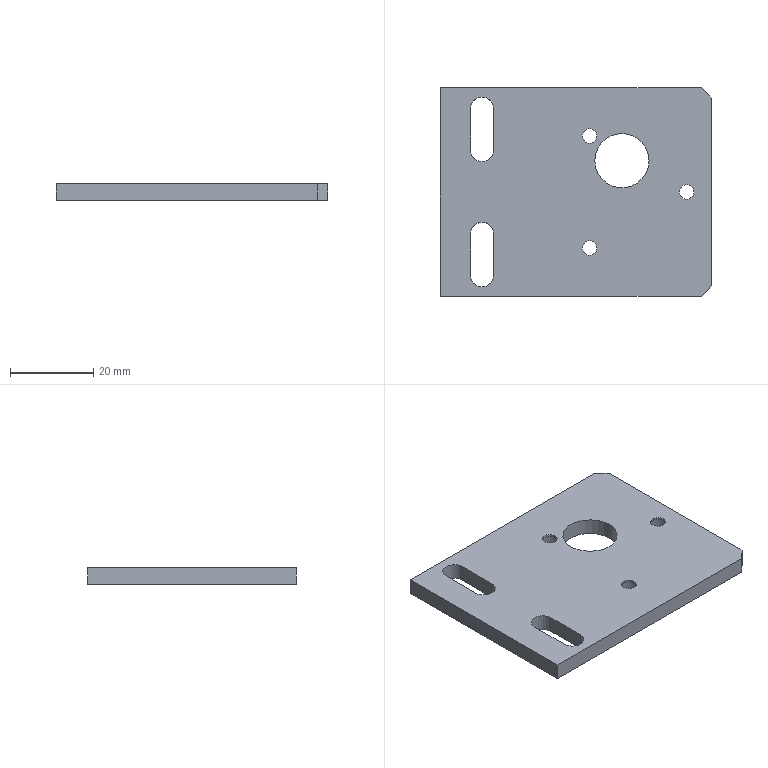Part | SolidWorks | features BaseBody 1 | 1 solid | 33 faces | box 65 x 50 x 4 mm | volume 11503 mm3 | cylinder 18 | plane 15 | commonest cylinder face diameters 3.5 x6 6 x6 5.5 x4 13 x2
STEP:
#1=CARTESIAN_POINT('',(41.797,20.428,0.));
#2=VERTEX_POINT('',#1);
#3=CARTESIAN_POINT('',(54.797,20.428,0.));
#4=VERTEX_POINT('',#3);
#5=CARTESIAN_POINT('',(48.297,20.428,0.));
#6=DIRECTION('',(0.,0.,1.));
#7=DIRECTION('',(1.,0.,0.));
#8=AXIS2_PLACEMENT_3D('',#5,#6,#7);
#9=CIRCLE('',#8,6.5);
#10=EDGE_CURVE('',#2,#4,#9,.T.);
#11=ORIENTED_EDGE('',*,*,#10,.F.);
#12=CARTESIAN_POINT('',(41.797,20.428,4.));
#13=VERTEX_POINT('',#12);
#14=CARTESIAN_POINT('',(41.797,20.428,-78.104));
#15=DIRECTION('',(0.,0.,1.));
#16=VECTOR('',#15,1000.);
#17=LINE('',#14,#16);
#18=EDGE_CURVE('',#2,#13,#17,.T.);
#19=ORIENTED_EDGE('',*,*,#18,.T.);
#20=CARTESIAN_POINT('',(54.797,20.428,4.));
#21=VERTEX_POINT('',#20);
#22=CARTESIAN_POINT('',(48.297,20.428,4.));
#23=DIRECTION('',(0.,0.,-1.));
#24=DIRECTION('',(1.,0.,0.));
#25=AXIS2_PLACEMENT_3D('',#22,#23,#24);
#26=CIRCLE('',#25,6.5);
#27=EDGE_CURVE('',#21,#13,#26,.T.);
#28=ORIENTED_EDGE('',*,*,#27,.F.);
#29=CARTESIAN_POINT('',(54.797,20.428,-78.104));
#30=DIRECTION('',(0.,0.,1.));
#31=VECTOR('',#30,1000.);
#32=LINE('',#29,#31);
#33=EDGE_CURVE('',#4,#21,#32,.T.);
#34=ORIENTED_EDGE('',*,*,#33,.F.);
#35=EDGE_LOOP('',(#11,#19,#28,#34));
#36=FACE_OUTER_BOUND('',#35,.T.);
#37=CARTESIAN_POINT('',(48.297,20.428,-78.104));
#38=DIRECTION('',(0.,0.,1.));
#39=DIRECTION('',(1.,0.,0.));
#40=AXIS2_PLACEMENT_3D('',#37,#38,#39);
#41=CYLINDRICAL_SURFACE('',#40,6.5);
#42=ADVANCED_FACE('',(#36),#41,.F.);
#43=CARTESIAN_POINT('',(42.297,26.328,4.));
#44=VERTEX_POINT('',#43);
#45=CARTESIAN_POINT('',(38.797,26.328,4.));
#46=VERTEX_POINT('',#45);
#47=CARTESIAN_POINT('',(40.547,26.328,4.));
#48=DIRECTION('',(0.,0.,-1.));
#49=DIRECTION('',(-1.,0.,0.));
#50=AXIS2_PLACEMENT_3D('',#47,#48,#49);
#51=CIRCLE('',#50,1.75);
#52=EDGE_CURVE('',#44,#46,#51,.T.);
#53=ORIENTED_EDGE('',*,*,#52,.F.);
#54=CARTESIAN_POINT('',(42.297,26.328,3.5));
#55=VERTEX_POINT('',#54);
#56=CARTESIAN_POINT('',(42.297,26.328,82.104));
#57=DIRECTION('',(0.,0.,-1.));
#58=VECTOR('',#57,1000.);
#59=LINE('',#56,#58);
#60=EDGE_CURVE('',#44,#55,#59,.T.);
#61=ORIENTED_EDGE('',*,*,#60,.T.);
#62=CARTESIAN_POINT('',(38.797,26.328,3.5));
#63=VERTEX_POINT('',#62);
#64=CARTESIAN_POINT('',(40.547,26.328,3.5));
#65=DIRECTION('',(0.,0.,1.));
#66=DIRECTION('',(-1.,0.,0.));
#67=AXIS2_PLACEMENT_3D('',#64,#65,#66);
#68=CIRCLE('',#67,1.75);
#69=EDGE_CURVE('',#63,#55,#68,.T.);
#70=ORIENTED_EDGE('',*,*,#69,.F.);
#71=CARTESIAN_POINT('',(38.797,26.328,82.104));
#72=DIRECTION('',(0.,0.,-1.));
#73=VECTOR('',#72,1000.);
#74=LINE('',#71,#73);
#75=EDGE_CURVE('',#46,#63,#74,.T.);
#76=ORIENTED_EDGE('',*,*,#75,.F.);
#77=EDGE_LOOP('',(#53,#61,#70,#76));
#78=FACE_OUTER_BOUND('',#77,.T.);
#79=CARTESIAN_POINT('',(40.547,26.328,82.104));
#80=DIRECTION('',(0.,0.,-1.));
#81=DIRECTION('',(-1.,0.,0.));
#82=AXIS2_PLACEMENT_3D('',#79,#80,#81);
#83=CYLINDRICAL_SURFACE('',#82,1.75);
#84=ADVANCED_FACE('',(#78),#83,.F.);
#85=CARTESIAN_POINT('',(42.297,-0.4722,4.));
#86=VERTEX_POINT('',#85);
#87=CARTESIAN_POINT('',(38.797,-0.4722,4.));
#88=VERTEX_POINT('',#87);
#89=CARTESIAN_POINT('',(40.547,-0.4722,4.));
#90=DIRECTION('',(0.,0.,-1.));
#91=DIRECTION('',(-1.,0.,0.));
#92=AXIS2_PLACEMENT_3D('',#89,#90,#91);
#93=CIRCLE('',#92,1.75);
#94=EDGE_CURVE('',#86,#88,#93,.T.);
#95=ORIENTED_EDGE('',*,*,#94,.F.);
#96=CARTESIAN_POINT('',(42.297,-0.4722,3.5));
#97=VERTEX_POINT('',#96);
#98=CARTESIAN_POINT('',(42.297,-0.4722,82.104));
#99=DIRECTION('',(0.,0.,-1.));
#100=VECTOR('',#99,1000.);
#101=LINE('',#98,#100);
#102=EDGE_CURVE('',#86,#97,#101,.T.);
#103=ORIENTED_EDGE('',*,*,#102,.T.);
#104=CARTESIAN_POINT('',(38.797,-0.4722,3.5));
#105=VERTEX_POINT('',#104);
#106=CARTESIAN_POINT('',(40.547,-0.4722,3.5));
#107=DIRECTION('',(0.,0.,1.));
#108=DIRECTION('',(-1.,0.,0.));
#109=AXIS2_PLACEMENT_3D('',#106,#107,#108);
#110=CIRCLE('',#109,1.75);
#111=EDGE_CURVE('',#105,#97,#110,.T.);
#112=ORIENTED_EDGE('',*,*,#111,.F.);
#113=CARTESIAN_POINT('',(38.797,-0.4722,82.104));
#114=DIRECTION('',(0.,0.,-1.));
#115=VECTOR('',#114,1000.);
#116=LINE('',#113,#115);
#117=EDGE_CURVE('',#88,#105,#116,.T.);
#118=ORIENTED_EDGE('',*,*,#117,.F.);
#119=EDGE_LOOP('',(#95,#103,#112,#118));
#120=FACE_OUTER_BOUND('',#119,.T.);
#121=CARTESIAN_POINT('',(40.547,-0.4722,82.104));
#122=DIRECTION('',(0.,0.,-1.));
#123=DIRECTION('',(-1.,0.,0.));
#124=AXIS2_PLACEMENT_3D('',#121,#122,#123);
#125=CYLINDRICAL_SURFACE('',#124,1.75);
#126=ADVANCED_FACE('',(#120),#125,.F.);
#127=CARTESIAN_POINT('',(65.547,12.928,4.));
#128=VERTEX_POINT('',#127);
#129=CARTESIAN_POINT('',(62.047,12.928,4.));
#130=VERTEX_POINT('',#129);
#131=CARTESIAN_POINT('',(63.797,12.928,4.));
#132=DIRECTION('',(0.,0.,-1.));
#133=DIRECTION('',(-1.,0.,0.));
#134=AXIS2_PLACEMENT_3D('',#131,#132,#133);
#135=CIRCLE('',#134,1.75);
#136=EDGE_CURVE('',#128,#130,#135,.T.);
#137=ORIENTED_EDGE('',*,*,#136,.F.);
#138=CARTESIAN_POINT('',(65.547,12.928,3.5));
#139=VERTEX_POINT('',#138);
#140=CARTESIAN_POINT('',(65.547,12.928,82.104));
#141=DIRECTION('',(0.,0.,-1.));
#142=VECTOR('',#141,1000.);
#143=LINE('',#140,#142);
#144=EDGE_CURVE('',#128,#139,#143,.T.);
#145=ORIENTED_EDGE('',*,*,#144,.T.);
#146=CARTESIAN_POINT('',(62.047,12.928,3.5));
#147=VERTEX_POINT('',#146);
#148=CARTESIAN_POINT('',(63.797,12.928,3.5));
#149=DIRECTION('',(0.,0.,1.));
#150=DIRECTION('',(-1.,0.,0.));
#151=AXIS2_PLACEMENT_3D('',#148,#149,#150);
#152=CIRCLE('',#151,1.75);
#153=EDGE_CURVE('',#147,#139,#152,.T.);
#154=ORIENTED_EDGE('',*,*,#153,.F.);
#155=CARTESIAN_POINT('',(62.047,12.928,82.104));
#156=DIRECTION('',(0.,0.,-1.));
#157=VECTOR('',#156,1000.);
#158=LINE('',#155,#157);
#159=EDGE_CURVE('',#130,#147,#158,.T.);
#160=ORIENTED_EDGE('',*,*,#159,.F.);
#161=EDGE_LOOP('',(#137,#145,#154,#160));
#162=FACE_OUTER_BOUND('',#161,.T.);
#163=CARTESIAN_POINT('',(63.797,12.928,82.104));
#164=DIRECTION('',(0.,0.,-1.));
#165=DIRECTION('',(-1.,0.,0.));
#166=AXIS2_PLACEMENT_3D('',#163,#164,#165);
#167=CYLINDRICAL_SURFACE('',#166,1.75);
#168=ADVANCED_FACE('',(#162),#167,.F.);
#169=CARTESIAN_POINT('',(43.547,26.328,3.5));
#170=VERTEX_POINT('',#169);
#171=CARTESIAN_POINT('',(37.547,26.328,3.5));
#172=VERTEX_POINT('',#171);
#173=CARTESIAN_POINT('',(40.547,26.328,3.5));
#174=DIRECTION('',(0.,0.,-1.));
#175=DIRECTION('',(-1.,0.,0.));
#176=AXIS2_PLACEMENT_3D('',#173,#174,#175);
#177=CIRCLE('',#176,3.);
#178=EDGE_CURVE('',#170,#172,#177,.T.);
#179=ORIENTED_EDGE('',*,*,#178,.F.);
#180=CARTESIAN_POINT('',(43.547,26.328,0.));
#181=VERTEX_POINT('',#180);
#182=CARTESIAN_POINT('',(43.547,26.328,1.75));
#183=DIRECTION('',(0.,0.,-1.));
#184=VECTOR('',#183,1000.);
#185=LINE('',#182,#184);
#186=EDGE_CURVE('',#170,#181,#185,.T.);
#187=ORIENTED_EDGE('',*,*,#186,.T.);
#188=CARTESIAN_POINT('',(37.547,26.328,0.));
#189=VERTEX_POINT('',#188);
#190=CARTESIAN_POINT('',(40.547,26.328,0.));
#191=DIRECTION('',(0.,0.,-1.));
#192=DIRECTION('',(-1.,0.,0.));
#193=AXIS2_PLACEMENT_3D('',#190,#191,#192);
#194=CIRCLE('',#193,3.);
#195=EDGE_CURVE('',#181,#189,#194,.T.);
#196=ORIENTED_EDGE('',*,*,#195,.T.);
#197=CARTESIAN_POINT('',(37.547,26.328,1.75));
#198=DIRECTION('',(0.,0.,-1.));
#199=VECTOR('',#198,1000.);
#200=LINE('',#197,#199);
#201=EDGE_CURVE('',#172,#189,#200,.T.);
#202=ORIENTED_EDGE('',*,*,#201,.F.);
#203=EDGE_LOOP('',(#179,#187,#196,#202));
#204=FACE_OUTER_BOUND('',#203,.T.);
#205=CARTESIAN_POINT('',(40.547,26.328,1.75));
#206=DIRECTION('',(0.,0.,-1.));
#207=DIRECTION('',(-1.,0.,0.));
#208=AXIS2_PLACEMENT_3D('',#205,#206,#207);
#209=CYLINDRICAL_SURFACE('',#208,3.);
#210=ADVANCED_FACE('',(#204),#209,.F.);
#211=CARTESIAN_POINT('',(43.547,-0.4722,3.5));
#212=VERTEX_POINT('',#211);
#213=CARTESIAN_POINT('',(37.547,-0.4722,3.5));
#214=VERTEX_POINT('',#213);
#215=CARTESIAN_POINT('',(40.547,-0.4722,3.5));
#216=DIRECTION('',(0.,0.,-1.));
#217=DIRECTION('',(-1.,0.,0.));
#218=AXIS2_PLACEMENT_3D('',#215,#216,#217);
#219=CIRCLE('',#218,3.);
#220=EDGE_CURVE('',#212,#214,#219,.T.);
#221=ORIENTED_EDGE('',*,*,#220,.F.);
#222=CARTESIAN_POINT('',(43.547,-0.4722,0.));
#223=VERTEX_POINT('',#222);
#224=CARTESIAN_POINT('',(43.547,-0.4722,1.75));
#225=DIRECTION('',(0.,0.,-1.));
#226=VECTOR('',#225,1000.);
#227=LINE('',#224,#226);
#228=EDGE_CURVE('',#212,#223,#227,.T.);
#229=ORIENTED_EDGE('',*,*,#228,.T.);
#230=CARTESIAN_POINT('',(37.547,-0.4722,0.));
#231=VERTEX_POINT('',#230);
#232=CARTESIAN_POINT('',(40.547,-0.4722,0.));
#233=DIRECTION('',(0.,0.,-1.));
#234=DIRECTION('',(-1.,0.,0.));
#235=AXIS2_PLACEMENT_3D('',#232,#233,#234);
#236=CIRCLE('',#235,3.);
#237=EDGE_CURVE('',#223,#231,#236,.T.);
#238=ORIENTED_EDGE('',*,*,#237,.T.);
#239=CARTESIAN_POINT('',(37.547,-0.4722,1.75));
#240=DIRECTION('',(0.,0.,-1.));
#241=VECTOR('',#240,1000.);
#242=LINE('',#239,#241);
#243=EDGE_CURVE('',#214,#231,#242,.T.);
#244=ORIENTED_EDGE('',*,*,#243,.F.);
#245=EDGE_LOOP('',(#221,#229,#238,#244));
#246=FACE_OUTER_BOUND('',#245,.T.);
#247=CARTESIAN_POINT('',(40.547,-0.4722,1.75));
#248=DIRECTION('',(0.,0.,-1.));
#249=DIRECTION('',(-1.,0.,0.));
#250=AXIS2_PLACEMENT_3D('',#247,#248,#249);
#251=CYLINDRICAL_SURFACE('',#250,3.);
#252=ADVANCED_FACE('',(#246),#251,.F.);
#253=CARTESIAN_POINT('',(66.797,12.928,3.5));
#254=VERTEX_POINT('',#253);
#255=CARTESIAN_POINT('',(60.797,12.928,3.5));
#256=VERTEX_POINT('',#255);
#257=CARTESIAN_POINT('',(63.797,12.928,3.5));
#258=DIRECTION('',(0.,0.,-1.));
#259=DIRECTION('',(-1.,0.,0.));
#260=AXIS2_PLACEMENT_3D('',#257,#258,#259);
#261=CIRCLE('',#260,3.);
#262=EDGE_CURVE('',#254,#256,#261,.T.);
#263=ORIENTED_EDGE('',*,*,#262,.F.);
#264=CARTESIAN_POINT('',(66.797,12.928,0.));
#265=VERTEX_POINT('',#264);
#266=CARTESIAN_POINT('',(66.797,12.928,1.75));
#267=DIRECTION('',(0.,0.,-1.));
#268=VECTOR('',#267,1000.);
#269=LINE('',#266,#268);
#270=EDGE_CURVE('',#254,#265,#269,.T.);
#271=ORIENTED_EDGE('',*,*,#270,.T.);
#272=CARTESIAN_POINT('',(60.797,12.928,0.));
#273=VERTEX_POINT('',#272);
#274=CARTESIAN_POINT('',(63.797,12.928,0.));
#275=DIRECTION('',(0.,0.,-1.));
#276=DIRECTION('',(-1.,0.,0.));
#277=AXIS2_PLACEMENT_3D('',#274,#275,#276);
#278=CIRCLE('',#277,3.);
#279=EDGE_CURVE('',#265,#273,#278,.T.);
#280=ORIENTED_EDGE('',*,*,#279,.T.);
#281=CARTESIAN_POINT('',(60.797,12.928,1.75));
#282=DIRECTION('',(0.,0.,-1.));
#283=VECTOR('',#282,1000.);
#284=LINE('',#281,#283);
#285=EDGE_CURVE('',#256,#273,#284,.T.);
#286=ORIENTED_EDGE('',*,*,#285,.F.);
#287=EDGE_LOOP('',(#263,#271,#280,#286));
#288=FACE_OUTER_BOUND('',#287,.T.);
#289=CARTESIAN_POINT('',(63.797,12.928,1.75));
#290=DIRECTION('',(0.,0.,-1.));
#291=DIRECTION('',(-1.,0.,0.));
#292=AXIS2_PLACEMENT_3D('',#289,#290,#291);
#293=CYLINDRICAL_SURFACE('',#292,3.);
#294=ADVANCED_FACE('',(#288),#293,.F.);
#295=CARTESIAN_POINT('',(17.547,32.928,4.));
#296=VERTEX_POINT('',#295);
#297=CARTESIAN_POINT('',(17.547,22.928,4.));
#298=VERTEX_POINT('',#297);
#299=CARTESIAN_POINT('',(17.547,12.928,4.));
#300=DIRECTION('',(0.,-1.,0.));
#301=VECTOR('',#300,1000.);
#302=LINE('',#299,#301);
#303=EDGE_CURVE('',#296,#298,#302,.T.);
#304=ORIENTED_EDGE('',*,*,#303,.T.);
#305=CARTESIAN_POINT('',(12.047,22.928,4.));
#306=VERTEX_POINT('',#305);
#307=CARTESIAN_POINT('',(14.797,22.928,4.));
#308=DIRECTION('',(0.,0.,-1.));
#309=DIRECTION('',(-1.,0.,0.));
#310=AXIS2_PLACEMENT_3D('',#307,#308,#309);
#311=CIRCLE('',#310,2.75);
#312=EDGE_CURVE('',#298,#306,#311,.T.);
#313=ORIENTED_EDGE('',*,*,#312,.T.);
#314=CARTESIAN_POINT('',(12.047,32.928,4.));
#315=VERTEX_POINT('',#314);
#316=CARTESIAN_POINT('',(12.047,12.928,4.));
#317=DIRECTION('',(0.,1.,0.));
#318=VECTOR('',#317,1000.);
#319=LINE('',#316,#318);
#320=EDGE_CURVE('',#306,#315,#319,.T.);
#321=ORIENTED_EDGE('',*,*,#320,.T.);
#322=CARTESIAN_POINT('',(14.797,32.928,4.));
#323=DIRECTION('',(0.,0.,-1.));
#324=DIRECTION('',(-1.,0.,0.));
#325=AXIS2_PLACEMENT_3D('',#322,#323,#324);
#326=CIRCLE('',#325,2.75);
#327=EDGE_CURVE('',#315,#296,#326,.T.);
#328=ORIENTED_EDGE('',*,*,#327,.T.);
#329=EDGE_LOOP('',(#304,#313,#321,#328));
#330=FACE_BOUND('',#329,.T.);
#331=CARTESIAN_POINT('',(17.547,2.928,4.));
#332=VERTEX_POINT('',#331);
#333=CARTESIAN_POINT('',(17.547,-7.072,4.));
#334=VERTEX_POINT('',#333);
#335=CARTESIAN_POINT('',(17.547,12.928,4.));
#336=DIRECTION('',(0.,-1.,0.));
#337=VECTOR('',#336,1000.);
#338=LINE('',#335,#337);
#339=EDGE_CURVE('',#332,#334,#338,.T.);
#340=ORIENTED_EDGE('',*,*,#339,.T.);
#341=CARTESIAN_POINT('',(12.047,-7.072,4.));
#342=VERTEX_POINT('',#341);
#343=CARTESIAN_POINT('',(14.797,-7.072,4.));
#344=DIRECTION('',(0.,0.,-1.));
#345=DIRECTION('',(-1.,0.,0.));
#346=AXIS2_PLACEMENT_3D('',#343,#344,#345);
#347=CIRCLE('',#346,2.75);
#348=EDGE_CURVE('',#334,#342,#347,.T.);
#349=ORIENTED_EDGE('',*,*,#348,.T.);
#350=CARTESIAN_POINT('',(12.047,2.928,4.));
#351=VERTEX_POINT('',#350);
#352=CARTESIAN_POINT('',(12.047,12.928,4.));
#353=DIRECTION('',(0.,1.,0.));
#354=VECTOR('',#353,1000.);
#355=LINE('',#352,#354);
#356=EDGE_CURVE('',#342,#351,#355,.T.);
#357=ORIENTED_EDGE('',*,*,#356,.T.);
#358=CARTESIAN_POINT('',(14.797,2.928,4.));
#359=DIRECTION('',(0.,0.,-1.));
#360=DIRECTION('',(-1.,0.,0.));
#361=AXIS2_PLACEMENT_3D('',#358,#359,#360);
#362=CIRCLE('',#361,2.75);
#363=EDGE_CURVE('',#351,#332,#362,.T.);
#364=ORIENTED_EDGE('',*,*,#363,.T.);
#365=EDGE_LOOP('',(#340,#349,#357,#364));
#366=FACE_BOUND('',#365,.T.);
#367=ORIENTED_EDGE('',*,*,#27,.T.);
#368=CARTESIAN_POINT('',(48.297,20.428,4.));
#369=DIRECTION('',(0.,0.,-1.));
#370=DIRECTION('',(1.,0.,0.));
#371=AXIS2_PLACEMENT_3D('',#368,#369,#370);
#372=CIRCLE('',#371,6.5);
#373=EDGE_CURVE('',#13,#21,#372,.T.);
#374=ORIENTED_EDGE('',*,*,#373,.T.);
#375=EDGE_LOOP('',(#367,#374));
#376=FACE_BOUND('',#375,.T.);
#377=CARTESIAN_POINT('',(40.547,26.328,4.));
#378=DIRECTION('',(0.,0.,-1.));
#379=DIRECTION('',(-1.,0.,0.));
#380=AXIS2_PLACEMENT_3D('',#377,#378,#379);
#381=CIRCLE('',#380,1.75);
#382=EDGE_CURVE('',#46,#44,#381,.T.);
#383=ORIENTED_EDGE('',*,*,#382,.T.);
#384=ORIENTED_EDGE('',*,*,#52,.T.);
#385=EDGE_LOOP('',(#383,#384));
#386=FACE_BOUND('',#385,.T.);
#387=CARTESIAN_POINT('',(40.547,-0.4722,4.));
#388=DIRECTION('',(0.,0.,-1.));
#389=DIRECTION('',(-1.,0.,0.));
#390=AXIS2_PLACEMENT_3D('',#387,#388,#389);
#391=CIRCLE('',#390,1.75);
#392=EDGE_CURVE('',#88,#86,#391,.T.);
#393=ORIENTED_EDGE('',*,*,#392,.T.);
#394=ORIENTED_EDGE('',*,*,#94,.T.);
#395=EDGE_LOOP('',(#393,#394));
#396=FACE_BOUND('',#395,.T.);
#397=CARTESIAN_POINT('',(63.797,12.928,4.));
#398=DIRECTION('',(0.,0.,-1.));
#399=DIRECTION('',(-1.,0.,0.));
#400=AXIS2_PLACEMENT_3D('',#397,#398,#399);
#401=CIRCLE('',#400,1.75);
#402=EDGE_CURVE('',#130,#128,#401,.T.);
#403=ORIENTED_EDGE('',*,*,#402,.T.);
#404=ORIENTED_EDGE('',*,*,#136,.T.);
#405=EDGE_LOOP('',(#403,#404));
#406=FACE_BOUND('',#405,.T.);
#407=CARTESIAN_POINT('',(4.797,37.928,4.));
#408=VERTEX_POINT('',#407);
#409=CARTESIAN_POINT('',(4.797,-12.072,4.));
#410=VERTEX_POINT('',#409);
#411=CARTESIAN_POINT('',(4.797,12.928,4.));
#412=DIRECTION('',(0.,-1.,0.));
#413=VECTOR('',#412,1000.);
#414=LINE('',#411,#413);
#415=EDGE_CURVE('',#408,#410,#414,.T.);
#416=ORIENTED_EDGE('',*,*,#415,.T.);
#417=CARTESIAN_POINT('',(67.297,-12.072,4.));
#418=VERTEX_POINT('',#417);
#419=CARTESIAN_POINT('',(37.297,-12.072,4.));
#420=DIRECTION('',(1.,0.,0.));
#421=VECTOR('',#420,1000.);
#422=LINE('',#419,#421);
#423=EDGE_CURVE('',#410,#418,#422,.T.);
#424=ORIENTED_EDGE('',*,*,#423,.T.);
#425=CARTESIAN_POINT('',(69.797,-9.572,4.));
#426=VERTEX_POINT('',#425);
#427=CARTESIAN_POINT('',(67.297,-12.072,4.));
#428=DIRECTION('',(0.7071,0.7071,0.));
#429=VECTOR('',#428,1000.);
#430=LINE('',#427,#429);
#431=EDGE_CURVE('',#418,#426,#430,.T.);
#432=ORIENTED_EDGE('',*,*,#431,.T.);
#433=CARTESIAN_POINT('',(69.797,35.428,4.));
#434=VERTEX_POINT('',#433);
#435=CARTESIAN_POINT('',(69.797,12.928,4.));
#436=DIRECTION('',(0.,1.,0.));
#437=VECTOR('',#436,1000.);
#438=LINE('',#435,#437);
#439=EDGE_CURVE('',#426,#434,#438,.T.);
#440=ORIENTED_EDGE('',*,*,#439,.T.);
#441=CARTESIAN_POINT('',(67.297,37.928,4.));
#442=VERTEX_POINT('',#441);
#443=CARTESIAN_POINT('',(69.797,35.428,4.));
#444=DIRECTION('',(-0.7071,0.7071,0.));
#445=VECTOR('',#444,1000.);
#446=LINE('',#443,#445);
#447=EDGE_CURVE('',#434,#442,#446,.T.);
#448=ORIENTED_EDGE('',*,*,#447,.T.);
#449=CARTESIAN_POINT('',(37.297,37.928,4.));
#450=DIRECTION('',(-1.,0.,0.));
#451=VECTOR('',#450,1000.);
#452=LINE('',#449,#451);
#453=EDGE_CURVE('',#442,#408,#452,.T.);
#454=ORIENTED_EDGE('',*,*,#453,.T.);
#455=EDGE_LOOP('',(#416,#424,#432,#440,#448,#454));
#456=FACE_OUTER_BOUND('',#455,.T.);
#457=CARTESIAN_POINT('',(37.297,12.928,4.));
#458=DIRECTION('',(0.,0.,1.));
#459=DIRECTION('',(1.,0.,0.));
#460=AXIS2_PLACEMENT_3D('',#457,#458,#459);
#461=PLANE('',#460);
#462=ADVANCED_FACE('',(#330,#366,#376,#386,#396,#406,#456),#461,.T.);
#463=CARTESIAN_POINT('',(12.047,22.928,0.));
#464=VERTEX_POINT('',#463);
#465=CARTESIAN_POINT('',(12.047,22.928,4.));
#466=DIRECTION('',(0.,0.,-1.));
#467=VECTOR('',#466,1000.);
#468=LINE('',#465,#467);
#469=EDGE_CURVE('',#306,#464,#468,.T.);
#470=ORIENTED_EDGE('',*,*,#469,.F.);
#471=ORIENTED_EDGE('',*,*,#312,.F.);
#472=CARTESIAN_POINT('',(17.547,22.928,0.));
#473=VERTEX_POINT('',#472);
#474=CARTESIAN_POINT('',(17.547,22.928,4.));
#475=DIRECTION('',(0.,0.,1.));
#476=VECTOR('',#475,1000.);
#477=LINE('',#474,#476);
#478=EDGE_CURVE('',#473,#298,#477,.T.);
#479=ORIENTED_EDGE('',*,*,#478,.F.);
#480=CARTESIAN_POINT('',(14.797,22.928,0.));
#481=DIRECTION('',(0.,0.,1.));
#482=DIRECTION('',(-1.,0.,0.));
#483=AXIS2_PLACEMENT_3D('',#480,#481,#482);
#484=CIRCLE('',#483,2.75);
#485=EDGE_CURVE('',#464,#473,#484,.T.);
#486=ORIENTED_EDGE('',*,*,#485,.F.);
#487=EDGE_LOOP('',(#470,#471,#479,#486));
#488=FACE_OUTER_BOUND('',#487,.T.);
#489=CARTESIAN_POINT('',(14.797,22.928,4.));
#490=DIRECTION('',(0.,0.,-1.));
#491=DIRECTION('',(-1.,0.,0.));
#492=AXIS2_PLACEMENT_3D('',#489,#490,#491);
#493=CYLINDRICAL_SURFACE('',#492,2.75);
#494=ADVANCED_FACE('',(#488),#493,.F.);
#495=ORIENTED_EDGE('',*,*,#478,.T.);
#496=ORIENTED_EDGE('',*,*,#303,.F.);
#497=CARTESIAN_POINT('',(17.547,32.928,0.));
#498=VERTEX_POINT('',#497);
#499=CARTESIAN_POINT('',(17.547,32.928,4.));
#500=DIRECTION('',(0.,0.,1.));
#501=VECTOR('',#500,1000.);
#502=LINE('',#499,#501);
#503=EDGE_CURVE('',#498,#296,#502,.T.);
#504=ORIENTED_EDGE('',*,*,#503,.F.);
#505=CARTESIAN_POINT('',(17.547,22.928,0.));
#506=DIRECTION('',(0.,1.,0.));
#507=VECTOR('',#506,1000.);
#508=LINE('',#505,#507);
#509=EDGE_CURVE('',#473,#498,#508,.T.);
#510=ORIENTED_EDGE('',*,*,#509,.F.);
#511=EDGE_LOOP('',(#495,#496,#504,#510));
#512=FACE_OUTER_BOUND('',#511,.T.);
#513=CARTESIAN_POINT('',(17.547,22.928,4.));
#514=DIRECTION('',(1.,0.,0.));
#515=DIRECTION('',(0.,0.,-1.));
#516=AXIS2_PLACEMENT_3D('',#513,#514,#515);
#517=PLANE('',#516);
#518=ADVANCED_FACE('',(#512),#517,.F.);
#519=ORIENTED_EDGE('',*,*,#503,.T.);
#520=ORIENTED_EDGE('',*,*,#327,.F.);
#521=CARTESIAN_POINT('',(12.047,32.928,0.));
#522=VERTEX_POINT('',#521);
#523=CARTESIAN_POINT('',(12.047,32.928,4.));
#524=DIRECTION('',(0.,0.,1.));
#525=VECTOR('',#524,1000.);
#526=LINE('',#523,#525);
#527=EDGE_CURVE('',#522,#315,#526,.T.);
#528=ORIENTED_EDGE('',*,*,#527,.F.);
#529=CARTESIAN_POINT('',(14.797,32.928,0.));
#530=DIRECTION('',(0.,0.,1.));
#531=DIRECTION('',(-1.,0.,0.));
#532=AXIS2_PLACEMENT_3D('',#529,#530,#531);
#533=CIRCLE('',#532,2.75);
#534=EDGE_CURVE('',#498,#522,#533,.T.);
#535=ORIENTED_EDGE('',*,*,#534,.F.);
#536=EDGE_LOOP('',(#519,#520,#528,#535));
#537=FACE_OUTER_BOUND('',#536,.T.);
#538=CARTESIAN_POINT('',(14.797,32.928,4.));
#539=DIRECTION('',(0.,0.,-1.));
#540=DIRECTION('',(-1.,0.,0.));
#541=AXIS2_PLACEMENT_3D('',#538,#539,#540);
#542=CYLINDRICAL_SURFACE('',#541,2.75);
#543=ADVANCED_FACE('',(#537),#542,.F.);
#544=ORIENTED_EDGE('',*,*,#527,.T.);
#545=ORIENTED_EDGE('',*,*,#320,.F.);
#546=ORIENTED_EDGE('',*,*,#469,.T.);
#547=CARTESIAN_POINT('',(12.047,32.928,0.));
#548=DIRECTION('',(0.,-1.,0.));
#549=VECTOR('',#548,1000.);
#550=LINE('',#547,#549);
#551=EDGE_CURVE('',#522,#464,#550,.T.);
#552=ORIENTED_EDGE('',*,*,#551,.F.);
#553=EDGE_LOOP('',(#544,#545,#546,#552));
#554=FACE_OUTER_BOUND('',#553,.T.);
#555=CARTESIAN_POINT('',(12.047,32.928,4.));
#556=DIRECTION('',(-1.,0.,0.));
#557=DIRECTION('',(0.,0.,1.));
#558=AXIS2_PLACEMENT_3D('',#555,#556,#557);
#559=PLANE('',#558);
#560=ADVANCED_FACE('',(#554),#559,.F.);
#561=CARTESIAN_POINT('',(12.047,-7.072,0.));
#562=VERTEX_POINT('',#561);
#563=CARTESIAN_POINT('',(12.047,-7.072,4.));
#564=DIRECTION('',(0.,0.,-1.));
#565=VECTOR('',#564,1000.);
#566=LINE('',#563,#565);
#567=EDGE_CURVE('',#342,#562,#566,.T.);
#568=ORIENTED_EDGE('',*,*,#567,.F.);
#569=ORIENTED_EDGE('',*,*,#348,.F.);
#570=CARTESIAN_POINT('',(17.547,-7.072,0.));
#571=VERTEX_POINT('',#570);
#572=CARTESIAN_POINT('',(17.547,-7.072,4.));
#573=DIRECTION('',(0.,0.,1.));
#574=VECTOR('',#573,1000.);
#575=LINE('',#572,#574);
#576=EDGE_CURVE('',#571,#334,#575,.T.);
#577=ORIENTED_EDGE('',*,*,#576,.F.);
#578=CARTESIAN_POINT('',(14.797,-7.072,0.));
#579=DIRECTION('',(0.,0.,1.));
#580=DIRECTION('',(-1.,0.,0.));
#581=AXIS2_PLACEMENT_3D('',#578,#579,#580);
#582=CIRCLE('',#581,2.75);
#583=EDGE_CURVE('',#562,#571,#582,.T.);
#584=ORIENTED_EDGE('',*,*,#583,.F.);
#585=EDGE_LOOP('',(#568,#569,#577,#584));
#586=FACE_OUTER_BOUND('',#585,.T.);
#587=CARTESIAN_POINT('',(14.797,-7.072,4.));
#588=DIRECTION('',(0.,0.,-1.));
#589=DIRECTION('',(-1.,0.,0.));
#590=AXIS2_PLACEMENT_3D('',#587,#588,#589);
#591=CYLINDRICAL_SURFACE('',#590,2.75);
#592=ADVANCED_FACE('',(#586),#591,.F.);
#593=ORIENTED_EDGE('',*,*,#576,.T.);
#594=ORIENTED_EDGE('',*,*,#339,.F.);
#595=CARTESIAN_POINT('',(17.547,2.928,0.));
#596=VERTEX_POINT('',#595);
#597=CARTESIAN_POINT('',(17.547,2.928,4.));
#598=DIRECTION('',(0.,0.,1.));
#599=VECTOR('',#598,1000.);
#600=LINE('',#597,#599);
#601=EDGE_CURVE('',#596,#332,#600,.T.);
#602=ORIENTED_EDGE('',*,*,#601,.F.);
#603=CARTESIAN_POINT('',(17.547,-7.072,0.));
#604=DIRECTION('',(0.,1.,0.));
#605=VECTOR('',#604,1000.);
#606=LINE('',#603,#605);
#607=EDGE_CURVE('',#571,#596,#606,.T.);
#608=ORIENTED_EDGE('',*,*,#607,.F.);
#609=EDGE_LOOP('',(#593,#594,#602,#608));
#610=FACE_OUTER_BOUND('',#609,.T.);
#611=CARTESIAN_POINT('',(17.547,-7.072,4.));
#612=DIRECTION('',(1.,0.,0.));
#613=DIRECTION('',(0.,0.,-1.));
#614=AXIS2_PLACEMENT_3D('',#611,#612,#613);
#615=PLANE('',#614);
#616=ADVANCED_FACE('',(#610),#615,.F.);
#617=ORIENTED_EDGE('',*,*,#601,.T.);
#618=ORIENTED_EDGE('',*,*,#363,.F.);
#619=CARTESIAN_POINT('',(12.047,2.928,0.));
#620=VERTEX_POINT('',#619);
#621=CARTESIAN_POINT('',(12.047,2.928,4.));
#622=DIRECTION('',(0.,0.,1.));
#623=VECTOR('',#622,1000.);
#624=LINE('',#621,#623);
#625=EDGE_CURVE('',#620,#351,#624,.T.);
#626=ORIENTED_EDGE('',*,*,#625,.F.);
#627=CARTESIAN_POINT('',(14.797,2.928,0.));
#628=DIRECTION('',(0.,0.,1.));
#629=DIRECTION('',(-1.,0.,0.));
#630=AXIS2_PLACEMENT_3D('',#627,#628,#629);
#631=CIRCLE('',#630,2.75);
#632=EDGE_CURVE('',#596,#620,#631,.T.);
#633=ORIENTED_EDGE('',*,*,#632,.F.);
#634=EDGE_LOOP('',(#617,#618,#626,#633));
#635=FACE_OUTER_BOUND('',#634,.T.);
#636=CARTESIAN_POINT('',(14.797,2.928,4.));
#637=DIRECTION('',(0.,0.,-1.));
#638=DIRECTION('',(-1.,0.,0.));
#639=AXIS2_PLACEMENT_3D('',#636,#637,#638);
#640=CYLINDRICAL_SURFACE('',#639,2.75);
#641=ADVANCED_FACE('',(#635),#640,.F.);
#642=ORIENTED_EDGE('',*,*,#625,.T.);
#643=ORIENTED_EDGE('',*,*,#356,.F.);
#644=ORIENTED_EDGE('',*,*,#567,.T.);
#645=CARTESIAN_POINT('',(12.047,2.928,0.));
#646=DIRECTION('',(0.,-1.,0.));
#647=VECTOR('',#646,1000.);
#648=LINE('',#645,#647);
#649=EDGE_CURVE('',#620,#562,#648,.T.);
#650=ORIENTED_EDGE('',*,*,#649,.F.);
#651=EDGE_LOOP('',(#642,#643,#644,#650));
#652=FACE_OUTER_BOUND('',#651,.T.);
#653=CARTESIAN_POINT('',(12.047,2.928,4.));
#654=DIRECTION('',(-1.,0.,0.));
#655=DIRECTION('',(0.,0.,1.));
#656=AXIS2_PLACEMENT_3D('',#653,#654,#655);
#657=PLANE('',#656);
#658=ADVANCED_FACE('',(#652),#657,.F.);
#659=ORIENTED_EDGE('',*,*,#18,.F.);
#660=CARTESIAN_POINT('',(48.297,20.428,0.));
#661=DIRECTION('',(0.,0.,1.));
#662=DIRECTION('',(1.,0.,0.));
#663=AXIS2_PLACEMENT_3D('',#660,#661,#662);
#664=CIRCLE('',#663,6.5);
#665=EDGE_CURVE('',#4,#2,#664,.T.);
#666=ORIENTED_EDGE('',*,*,#665,.F.);
#667=ORIENTED_EDGE('',*,*,#33,.T.);
#668=ORIENTED_EDGE('',*,*,#373,.F.);
#669=EDGE_LOOP('',(#659,#666,#667,#668));
#670=FACE_OUTER_BOUND('',#669,.T.);
#671=CARTESIAN_POINT('',(48.297,20.428,-78.104));
#672=DIRECTION('',(0.,0.,1.));
#673=DIRECTION('',(1.,0.,0.));
#674=AXIS2_PLACEMENT_3D('',#671,#672,#673);
#675=CYLINDRICAL_SURFACE('',#674,6.5);
#676=ADVANCED_FACE('',(#670),#675,.F.);
#677=ORIENTED_EDGE('',*,*,#60,.F.);
#678=ORIENTED_EDGE('',*,*,#382,.F.);
#679=ORIENTED_EDGE('',*,*,#75,.T.);
#680=CARTESIAN_POINT('',(40.547,26.328,3.5));
#681=DIRECTION('',(0.,0.,1.));
#682=DIRECTION('',(-1.,0.,0.));
#683=AXIS2_PLACEMENT_3D('',#680,#681,#682);
#684=CIRCLE('',#683,1.75);
#685=EDGE_CURVE('',#55,#63,#684,.T.);
#686=ORIENTED_EDGE('',*,*,#685,.F.);
#687=EDGE_LOOP('',(#677,#678,#679,#686));
#688=FACE_OUTER_BOUND('',#687,.T.);
#689=CARTESIAN_POINT('',(40.547,26.328,82.104));
#690=DIRECTION('',(0.,0.,-1.));
#691=DIRECTION('',(-1.,0.,0.));
#692=AXIS2_PLACEMENT_3D('',#689,#690,#691);
#693=CYLINDRICAL_SURFACE('',#692,1.75);
#694=ADVANCED_FACE('',(#688),#693,.F.);
#695=ORIENTED_EDGE('',*,*,#102,.F.);
#696=ORIENTED_EDGE('',*,*,#392,.F.);
#697=ORIENTED_EDGE('',*,*,#117,.T.);
#698=CARTESIAN_POINT('',(40.547,-0.4722,3.5));
#699=DIRECTION('',(0.,0.,1.));
#700=DIRECTION('',(-1.,0.,0.));
#701=AXIS2_PLACEMENT_3D('',#698,#699,#700);
#702=CIRCLE('',#701,1.75);
#703=EDGE_CURVE('',#97,#105,#702,.T.);
#704=ORIENTED_EDGE('',*,*,#703,.F.);
#705=EDGE_LOOP('',(#695,#696,#697,#704));
#706=FACE_OUTER_BOUND('',#705,.T.);
#707=CARTESIAN_POINT('',(40.547,-0.4722,82.104));
#708=DIRECTION('',(0.,0.,-1.));
#709=DIRECTION('',(-1.,0.,0.));
#710=AXIS2_PLACEMENT_3D('',#707,#708,#709);
#711=CYLINDRICAL_SURFACE('',#710,1.75);
#712=ADVANCED_FACE('',(#706),#711,.F.);
#713=ORIENTED_EDGE('',*,*,#144,.F.);
#714=ORIENTED_EDGE('',*,*,#402,.F.);
#715=ORIENTED_EDGE('',*,*,#159,.T.);
#716=CARTESIAN_POINT('',(63.797,12.928,3.5));
#717=DIRECTION('',(0.,0.,1.));
#718=DIRECTION('',(-1.,0.,0.));
#719=AXIS2_PLACEMENT_3D('',#716,#717,#718);
#720=CIRCLE('',#719,1.75);
#721=EDGE_CURVE('',#139,#147,#720,.T.);
#722=ORIENTED_EDGE('',*,*,#721,.F.);
#723=EDGE_LOOP('',(#713,#714,#715,#722));
#724=FACE_OUTER_BOUND('',#723,.T.);
#725=CARTESIAN_POINT('',(63.797,12.928,82.104));
#726=DIRECTION('',(0.,0.,-1.));
#727=DIRECTION('',(-1.,0.,0.));
#728=AXIS2_PLACEMENT_3D('',#725,#726,#727);
#729=CYLINDRICAL_SURFACE('',#728,1.75);
#730=ADVANCED_FACE('',(#724),#729,.F.);
#731=CARTESIAN_POINT('',(4.797,-12.072,0.));
#732=VERTEX_POINT('',#731);
#733=CARTESIAN_POINT('',(4.797,-12.072,0.));
#734=DIRECTION('',(0.,0.,-1.));
#735=VECTOR('',#734,1000.);
#736=LINE('',#733,#735);
#737=EDGE_CURVE('',#410,#732,#736,.T.);
#738=ORIENTED_EDGE('',*,*,#737,.T.);
#739=CARTESIAN_POINT('',(67.297,-12.072,0.));
#740=VERTEX_POINT('',#739);
#741=CARTESIAN_POINT('',(69.797,-12.072,0.));
#742=DIRECTION('',(1.,0.,0.));
#743=VECTOR('',#742,1000.);
#744=LINE('',#741,#743);
#745=EDGE_CURVE('',#732,#740,#744,.T.);
#746=ORIENTED_EDGE('',*,*,#745,.T.);
#747=CARTESIAN_POINT('',(67.297,-12.072,0.));
#748=DIRECTION('',(0.,0.,1.));
#749=VECTOR('',#748,1000.);
#750=LINE('',#747,#749);
#751=EDGE_CURVE('',#740,#418,#750,.T.);
#752=ORIENTED_EDGE('',*,*,#751,.T.);
#753=ORIENTED_EDGE('',*,*,#423,.F.);
#754=EDGE_LOOP('',(#738,#746,#752,#753));
#755=FACE_OUTER_BOUND('',#754,.T.);
#756=CARTESIAN_POINT('',(69.797,-12.072,0.));
#757=DIRECTION('',(0.,-1.,0.));
#758=DIRECTION('',(0.,0.,-1.));
#759=AXIS2_PLACEMENT_3D('',#756,#757,#758);
#760=PLANE('',#759);
#761=ADVANCED_FACE('',(#755),#760,.T.);
#762=CARTESIAN_POINT('',(4.797,37.928,0.));
#763=VERTEX_POINT('',#762);
#764=CARTESIAN_POINT('',(4.797,-12.072,0.));
#765=DIRECTION('',(0.,-1.,0.));
#766=VECTOR('',#765,1000.);
#767=LINE('',#764,#766);
#768=EDGE_CURVE('',#763,#732,#767,.T.);
#769=ORIENTED_EDGE('',*,*,#768,.T.);
#770=ORIENTED_EDGE('',*,*,#737,.F.);
#771=ORIENTED_EDGE('',*,*,#415,.F.);
#772=CARTESIAN_POINT('',(4.797,37.928,0.));
#773=DIRECTION('',(0.,0.,-1.));
#774=VECTOR('',#773,1000.);
#775=LINE('',#772,#774);
#776=EDGE_CURVE('',#408,#763,#775,.T.);
#777=ORIENTED_EDGE('',*,*,#776,.T.);
#778=EDGE_LOOP('',(#769,#770,#771,#777));
#779=FACE_OUTER_BOUND('',#778,.T.);
#780=CARTESIAN_POINT('',(4.797,-12.072,0.));
#781=DIRECTION('',(-1.,0.,0.));
#782=DIRECTION('',(0.,0.,1.));
#783=AXIS2_PLACEMENT_3D('',#780,#781,#782);
#784=PLANE('',#783);
#785=ADVANCED_FACE('',(#779),#784,.T.);
#786=ORIENTED_EDGE('',*,*,#776,.F.);
#787=ORIENTED_EDGE('',*,*,#453,.F.);
#788=CARTESIAN_POINT('',(67.297,37.928,0.));
#789=VERTEX_POINT('',#788);
#790=CARTESIAN_POINT('',(67.297,37.928,0.));
#791=DIRECTION('',(0.,0.,-1.));
#792=VECTOR('',#791,1000.);
#793=LINE('',#790,#792);
#794=EDGE_CURVE('',#442,#789,#793,.T.);
#795=ORIENTED_EDGE('',*,*,#794,.T.);
#796=CARTESIAN_POINT('',(4.797,37.928,0.));
#797=DIRECTION('',(-1.,0.,0.));
#798=VECTOR('',#797,1000.);
#799=LINE('',#796,#798);
#800=EDGE_CURVE('',#789,#763,#799,.T.);
#801=ORIENTED_EDGE('',*,*,#800,.T.);
#802=EDGE_LOOP('',(#786,#787,#795,#801));
#803=FACE_OUTER_BOUND('',#802,.T.);
#804=CARTESIAN_POINT('',(4.797,37.928,0.));
#805=DIRECTION('',(0.,1.,0.));
#806=DIRECTION('',(0.,0.,1.));
#807=AXIS2_PLACEMENT_3D('',#804,#805,#806);
#808=PLANE('',#807);
#809=ADVANCED_FACE('',(#803),#808,.T.);
#810=CARTESIAN_POINT('',(69.797,35.428,0.));
#811=VERTEX_POINT('',#810);
#812=CARTESIAN_POINT('',(68.547,36.678,0.));
#813=DIRECTION('',(-0.7071,0.7071,0.));
#814=VECTOR('',#813,1000.);
#815=LINE('',#812,#814);
#816=EDGE_CURVE('',#811,#789,#815,.T.);
#817=ORIENTED_EDGE('',*,*,#816,.T.);
#818=ORIENTED_EDGE('',*,*,#794,.F.);
#819=ORIENTED_EDGE('',*,*,#447,.F.);
#820=CARTESIAN_POINT('',(69.797,35.428,0.));
#821=DIRECTION('',(0.,0.,-1.));
#822=VECTOR('',#821,1000.);
#823=LINE('',#820,#822);
#824=EDGE_CURVE('',#434,#811,#823,.T.);
#825=ORIENTED_EDGE('',*,*,#824,.T.);
#826=EDGE_LOOP('',(#817,#818,#819,#825));
#827=FACE_OUTER_BOUND('',#826,.T.);
#828=CARTESIAN_POINT('',(68.547,36.678,0.));
#829=DIRECTION('',(0.7071,0.7071,0.));
#830=DIRECTION('',(-0.7071,0.7071,0.));
#831=AXIS2_PLACEMENT_3D('',#828,#829,#830);
#832=PLANE('',#831);
#833=ADVANCED_FACE('',(#827),#832,.T.);
#834=ORIENTED_EDGE('',*,*,#824,.F.);
#835=ORIENTED_EDGE('',*,*,#439,.F.);
#836=CARTESIAN_POINT('',(69.797,-9.572,0.));
#837=VERTEX_POINT('',#836);
#838=CARTESIAN_POINT('',(69.797,-9.572,0.));
#839=DIRECTION('',(0.,0.,-1.));
#840=VECTOR('',#839,1000.);
#841=LINE('',#838,#840);
#842=EDGE_CURVE('',#426,#837,#841,.T.);
#843=ORIENTED_EDGE('',*,*,#842,.T.);
#844=CARTESIAN_POINT('',(69.797,37.928,0.));
#845=DIRECTION('',(0.,1.,0.));
#846=VECTOR('',#845,1000.);
#847=LINE('',#844,#846);
#848=EDGE_CURVE('',#837,#811,#847,.T.);
#849=ORIENTED_EDGE('',*,*,#848,.T.);
#850=EDGE_LOOP('',(#834,#835,#843,#849));
#851=FACE_OUTER_BOUND('',#850,.T.);
#852=CARTESIAN_POINT('',(69.797,37.928,0.));
#853=DIRECTION('',(1.,0.,0.));
#854=DIRECTION('',(0.,0.,-1.));
#855=AXIS2_PLACEMENT_3D('',#852,#853,#854);
#856=PLANE('',#855);
#857=ADVANCED_FACE('',(#851),#856,.T.);
#858=CARTESIAN_POINT('',(68.547,-10.822,0.));
#859=DIRECTION('',(0.7071,0.7071,0.));
#860=VECTOR('',#859,1000.);
#861=LINE('',#858,#860);
#862=EDGE_CURVE('',#740,#837,#861,.T.);
#863=ORIENTED_EDGE('',*,*,#862,.T.);
#864=ORIENTED_EDGE('',*,*,#842,.F.);
#865=ORIENTED_EDGE('',*,*,#431,.F.);
#866=ORIENTED_EDGE('',*,*,#751,.F.);
#867=EDGE_LOOP('',(#863,#864,#865,#866));
#868=FACE_OUTER_BOUND('',#867,.T.);
#869=CARTESIAN_POINT('',(68.547,-10.822,0.));
#870=DIRECTION('',(0.7071,-0.7071,0.));
#871=DIRECTION('',(0.7071,0.7071,0.));
#872=AXIS2_PLACEMENT_3D('',#869,#870,#871);
#873=PLANE('',#872);
#874=ADVANCED_FACE('',(#868),#873,.T.);
#875=ORIENTED_EDGE('',*,*,#485,.T.);
#876=ORIENTED_EDGE('',*,*,#509,.T.);
#877=ORIENTED_EDGE('',*,*,#534,.T.);
#878=ORIENTED_EDGE('',*,*,#551,.T.);
#879=EDGE_LOOP('',(#875,#876,#877,#878));
#880=FACE_BOUND('',#879,.T.);
#881=ORIENTED_EDGE('',*,*,#583,.T.);
#882=ORIENTED_EDGE('',*,*,#607,.T.);
#883=ORIENTED_EDGE('',*,*,#632,.T.);
#884=ORIENTED_EDGE('',*,*,#649,.T.);
#885=EDGE_LOOP('',(#881,#882,#883,#884));
#886=FACE_BOUND('',#885,.T.);
#887=ORIENTED_EDGE('',*,*,#665,.T.);
#888=ORIENTED_EDGE('',*,*,#10,.T.);
#889=EDGE_LOOP('',(#887,#888));
#890=FACE_BOUND('',#889,.T.);
#891=CARTESIAN_POINT('',(40.547,26.328,0.));
#892=DIRECTION('',(0.,0.,-1.));
#893=DIRECTION('',(-1.,0.,0.));
#894=AXIS2_PLACEMENT_3D('',#891,#892,#893);
#895=CIRCLE('',#894,3.);
#896=EDGE_CURVE('',#189,#181,#895,.T.);
#897=ORIENTED_EDGE('',*,*,#896,.F.);
#898=ORIENTED_EDGE('',*,*,#195,.F.);
#899=EDGE_LOOP('',(#897,#898));
#900=FACE_BOUND('',#899,.T.);
#901=CARTESIAN_POINT('',(40.547,-0.4722,0.));
#902=DIRECTION('',(0.,0.,-1.));
#903=DIRECTION('',(-1.,0.,0.));
#904=AXIS2_PLACEMENT_3D('',#901,#902,#903);
#905=CIRCLE('',#904,3.);
#906=EDGE_CURVE('',#231,#223,#905,.T.);
#907=ORIENTED_EDGE('',*,*,#906,.F.);
#908=ORIENTED_EDGE('',*,*,#237,.F.);
#909=EDGE_LOOP('',(#907,#908));
#910=FACE_BOUND('',#909,.T.);
#911=CARTESIAN_POINT('',(63.797,12.928,0.));
#912=DIRECTION('',(0.,0.,-1.));
#913=DIRECTION('',(-1.,0.,0.));
#914=AXIS2_PLACEMENT_3D('',#911,#912,#913);
#915=CIRCLE('',#914,3.);
#916=EDGE_CURVE('',#273,#265,#915,.T.);
#917=ORIENTED_EDGE('',*,*,#916,.F.);
#918=ORIENTED_EDGE('',*,*,#279,.F.);
#919=EDGE_LOOP('',(#917,#918));
#920=FACE_BOUND('',#919,.T.);
#921=ORIENTED_EDGE('',*,*,#745,.F.);
#922=ORIENTED_EDGE('',*,*,#768,.F.);
#923=ORIENTED_EDGE('',*,*,#800,.F.);
#924=ORIENTED_EDGE('',*,*,#816,.F.);
#925=ORIENTED_EDGE('',*,*,#848,.F.);
#926=ORIENTED_EDGE('',*,*,#862,.F.);
#927=EDGE_LOOP('',(#921,#922,#923,#924,#925,#926));
#928=FACE_OUTER_BOUND('',#927,.T.);
#929=CARTESIAN_POINT('',(37.297,12.928,0.));
#930=DIRECTION('',(0.,0.,1.));
#931=DIRECTION('',(1.,0.,0.));
#932=AXIS2_PLACEMENT_3D('',#929,#930,#931);
#933=PLANE('',#932);
#934=ADVANCED_FACE('',(#880,#886,#890,#900,#910,#920,#928),#933,.F.);
#935=ORIENTED_EDGE('',*,*,#69,.T.);
#936=ORIENTED_EDGE('',*,*,#685,.T.);
#937=EDGE_LOOP('',(#935,#936));
#938=FACE_BOUND('',#937,.T.);
#939=CARTESIAN_POINT('',(40.547,26.328,3.5));
#940=DIRECTION('',(0.,0.,-1.));
#941=DIRECTION('',(-1.,0.,0.));
#942=AXIS2_PLACEMENT_3D('',#939,#940,#941);
#943=CIRCLE('',#942,3.);
#944=EDGE_CURVE('',#172,#170,#943,.T.);
#945=ORIENTED_EDGE('',*,*,#944,.T.);
#946=ORIENTED_EDGE('',*,*,#178,.T.);
#947=EDGE_LOOP('',(#945,#946));
#948=FACE_OUTER_BOUND('',#947,.T.);
#949=CARTESIAN_POINT('',(40.547,26.328,3.5));
#950=DIRECTION('',(0.,0.,-1.));
#951=DIRECTION('',(-1.,0.,0.));
#952=AXIS2_PLACEMENT_3D('',#949,#950,#951);
#953=PLANE('',#952);
#954=ADVANCED_FACE('',(#938,#948),#953,.T.);
#955=ORIENTED_EDGE('',*,*,#111,.T.);
#956=ORIENTED_EDGE('',*,*,#703,.T.);
#957=EDGE_LOOP('',(#955,#956));
#958=FACE_BOUND('',#957,.T.);
#959=CARTESIAN_POINT('',(40.547,-0.4722,3.5));
#960=DIRECTION('',(0.,0.,-1.));
#961=DIRECTION('',(-1.,0.,0.));
#962=AXIS2_PLACEMENT_3D('',#959,#960,#961);
#963=CIRCLE('',#962,3.);
#964=EDGE_CURVE('',#214,#212,#963,.T.);
#965=ORIENTED_EDGE('',*,*,#964,.T.);
#966=ORIENTED_EDGE('',*,*,#220,.T.);
#967=EDGE_LOOP('',(#965,#966));
#968=FACE_OUTER_BOUND('',#967,.T.);
#969=CARTESIAN_POINT('',(40.547,-0.4722,3.5));
#970=DIRECTION('',(0.,0.,-1.));
#971=DIRECTION('',(-1.,0.,0.));
#972=AXIS2_PLACEMENT_3D('',#969,#970,#971);
#973=PLANE('',#972);
#974=ADVANCED_FACE('',(#958,#968),#973,.T.);
#975=ORIENTED_EDGE('',*,*,#153,.T.);
#976=ORIENTED_EDGE('',*,*,#721,.T.);
#977=EDGE_LOOP('',(#975,#976));
#978=FACE_BOUND('',#977,.T.);
#979=CARTESIAN_POINT('',(63.797,12.928,3.5));
#980=DIRECTION('',(0.,0.,-1.));
#981=DIRECTION('',(-1.,0.,0.));
#982=AXIS2_PLACEMENT_3D('',#979,#980,#981);
#983=CIRCLE('',#982,3.);
#984=EDGE_CURVE('',#256,#254,#983,.T.);
#985=ORIENTED_EDGE('',*,*,#984,.T.);
#986=ORIENTED_EDGE('',*,*,#262,.T.);
#987=EDGE_LOOP('',(#985,#986));
#988=FACE_OUTER_BOUND('',#987,.T.);
#989=CARTESIAN_POINT('',(63.797,12.928,3.5));
#990=DIRECTION('',(0.,0.,-1.));
#991=DIRECTION('',(-1.,0.,0.));
#992=AXIS2_PLACEMENT_3D('',#989,#990,#991);
#993=PLANE('',#992);
#994=ADVANCED_FACE('',(#978,#988),#993,.T.);
#995=ORIENTED_EDGE('',*,*,#186,.F.);
#996=ORIENTED_EDGE('',*,*,#944,.F.);
#997=ORIENTED_EDGE('',*,*,#201,.T.);
#998=ORIENTED_EDGE('',*,*,#896,.T.);
#999=EDGE_LOOP('',(#995,#996,#997,#998));
#1000=FACE_OUTER_BOUND('',#999,.T.);
#1001=CARTESIAN_POINT('',(40.547,26.328,1.75));
#1002=DIRECTION('',(0.,0.,-1.));
#1003=DIRECTION('',(-1.,0.,0.));
#1004=AXIS2_PLACEMENT_3D('',#1001,#1002,#1003);
#1005=CYLINDRICAL_SURFACE('',#1004,3.);
#1006=ADVANCED_FACE('',(#1000),#1005,.F.);
#1007=ORIENTED_EDGE('',*,*,#228,.F.);
#1008=ORIENTED_EDGE('',*,*,#964,.F.);
#1009=ORIENTED_EDGE('',*,*,#243,.T.);
#1010=ORIENTED_EDGE('',*,*,#906,.T.);
#1011=EDGE_LOOP('',(#1007,#1008,#1009,#1010));
#1012=FACE_OUTER_BOUND('',#1011,.T.);
#1013=CARTESIAN_POINT('',(40.547,-0.4722,1.75));
#1014=DIRECTION('',(0.,0.,-1.));
#1015=DIRECTION('',(-1.,0.,0.));
#1016=AXIS2_PLACEMENT_3D('',#1013,#1014,#1015);
#1017=CYLINDRICAL_SURFACE('',#1016,3.);
#1018=ADVANCED_FACE('',(#1012),#1017,.F.);
#1019=ORIENTED_EDGE('',*,*,#270,.F.);
#1020=ORIENTED_EDGE('',*,*,#984,.F.);
#1021=ORIENTED_EDGE('',*,*,#285,.T.);
#1022=ORIENTED_EDGE('',*,*,#916,.T.);
#1023=EDGE_LOOP('',(#1019,#1020,#1021,#1022));
#1024=FACE_OUTER_BOUND('',#1023,.T.);
#1025=CARTESIAN_POINT('',(63.797,12.928,1.75));
#1026=DIRECTION('',(0.,0.,-1.));
#1027=DIRECTION('',(-1.,0.,0.));
#1028=AXIS2_PLACEMENT_3D('',#1025,#1026,#1027);
#1029=CYLINDRICAL_SURFACE('',#1028,3.);
#1030=ADVANCED_FACE('',(#1024),#1029,.F.);
#1031=CLOSED_SHELL('',(#42,#84,#126,#168,#210,#252,#294,#462,#494,#518,#543,#560,#592,#616,#641,#658,#676,#694,#712,#730,#761,#785,#809,#833,#857,#874,#934,#954,#974,#994,#1006,#1018,#1030));
#1032=MANIFOLD_SOLID_BREP('',#1031);
#1033=CARTESIAN_POINT('',(0.,0.,0.));
#1034=DIRECTION('',(0.,0.,1.));
#1035=DIRECTION('',(1.,0.,0.));
#1036=AXIS2_PLACEMENT_3D('',#1033,#1034,#1035);
#1037=(LENGTH_UNIT()NAMED_UNIT(*)SI_UNIT(.MILLI.,.METRE.));
#1038=UNCERTAINTY_MEASURE_WITH_UNIT(LENGTH_MEASURE(0.00001),#1037,'','');
#1039=(NAMED_UNIT(*)PLANE_ANGLE_UNIT()SI_UNIT($,.RADIAN.));
#1040=(NAMED_UNIT(*)SI_UNIT($,.STERADIAN.)SOLID_ANGLE_UNIT());
#1041=(GEOMETRIC_REPRESENTATION_CONTEXT(3)GLOBAL_UNCERTAINTY_ASSIGNED_CONTEXT((#1038))GLOBAL_UNIT_ASSIGNED_CONTEXT((#1037,#1039,#1040))REPRESENTATION_CONTEXT('',''));
#1042=ADVANCED_BREP_SHAPE_REPRESENTATION('',(#1032,#1036),#1041);